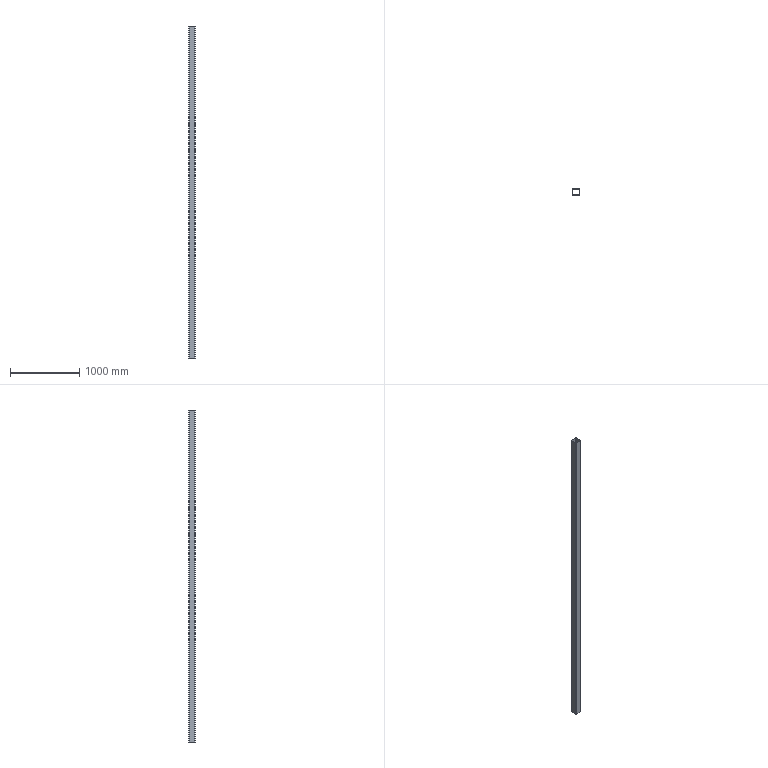Part | SolidWorks | features Extrusion 1 | 1 solid | 18 faces | box 100 x 100 x 4800 mm | volume 8810973 mm3 | plane 10 | cylinder 8 | commonest cylinder face diameters 10 x4 20 x4
STEP:
#1=CARTESIAN_POINT('',(-40.,50.,2400.));
#2=VERTEX_POINT('',#1);
#3=CARTESIAN_POINT('',(-50.,40.,2400.));
#4=VERTEX_POINT('',#3);
#5=CARTESIAN_POINT('',(-40.,40.,2400.));
#6=DIRECTION('',(0.,0.,1.));
#7=DIRECTION('',(1.,0.,0.));
#8=AXIS2_PLACEMENT_3D('',#5,#6,#7);
#9=CIRCLE('',#8,10.);
#10=EDGE_CURVE('',#2,#4,#9,.T.);
#11=ORIENTED_EDGE('',*,*,#10,.T.);
#12=CARTESIAN_POINT('',(-50.,-40.,2400.));
#13=VERTEX_POINT('',#12);
#14=CARTESIAN_POINT('',(-50.,40.,2400.));
#15=DIRECTION('',(0.,-1.,0.));
#16=VECTOR('',#15,1000.);
#17=LINE('',#14,#16);
#18=EDGE_CURVE('',#4,#13,#17,.T.);
#19=ORIENTED_EDGE('',*,*,#18,.T.);
#20=CARTESIAN_POINT('',(-40.,-50.,2400.));
#21=VERTEX_POINT('',#20);
#22=CARTESIAN_POINT('',(-40.,-40.,2400.));
#23=DIRECTION('',(0.,0.,1.));
#24=DIRECTION('',(-1.,0.,0.));
#25=AXIS2_PLACEMENT_3D('',#22,#23,#24);
#26=CIRCLE('',#25,10.);
#27=EDGE_CURVE('',#13,#21,#26,.T.);
#28=ORIENTED_EDGE('',*,*,#27,.T.);
#29=CARTESIAN_POINT('',(40.,-50.,2400.));
#30=VERTEX_POINT('',#29);
#31=CARTESIAN_POINT('',(40.,-50.,2400.));
#32=DIRECTION('',(1.,0.,0.));
#33=VECTOR('',#32,1000.);
#34=LINE('',#31,#33);
#35=EDGE_CURVE('',#21,#30,#34,.T.);
#36=ORIENTED_EDGE('',*,*,#35,.T.);
#37=CARTESIAN_POINT('',(50.,-40.,2400.));
#38=VERTEX_POINT('',#37);
#39=CARTESIAN_POINT('',(40.,-40.,2400.));
#40=DIRECTION('',(0.,0.,1.));
#41=DIRECTION('',(1.,0.,0.));
#42=AXIS2_PLACEMENT_3D('',#39,#40,#41);
#43=CIRCLE('',#42,10.);
#44=EDGE_CURVE('',#30,#38,#43,.T.);
#45=ORIENTED_EDGE('',*,*,#44,.T.);
#46=CARTESIAN_POINT('',(50.,40.,2400.));
#47=VERTEX_POINT('',#46);
#48=CARTESIAN_POINT('',(50.,-40.,2400.));
#49=DIRECTION('',(0.,1.,0.));
#50=VECTOR('',#49,1000.);
#51=LINE('',#48,#50);
#52=EDGE_CURVE('',#38,#47,#51,.T.);
#53=ORIENTED_EDGE('',*,*,#52,.T.);
#54=CARTESIAN_POINT('',(40.,50.,2400.));
#55=VERTEX_POINT('',#54);
#56=CARTESIAN_POINT('',(40.,40.,2400.));
#57=DIRECTION('',(0.,0.,1.));
#58=DIRECTION('',(-1.,0.,0.));
#59=AXIS2_PLACEMENT_3D('',#56,#57,#58);
#60=CIRCLE('',#59,10.);
#61=EDGE_CURVE('',#47,#55,#60,.T.);
#62=ORIENTED_EDGE('',*,*,#61,.T.);
#63=CARTESIAN_POINT('',(0.,50.,2400.));
#64=DIRECTION('',(-1.,0.,0.));
#65=VECTOR('',#64,1000.);
#66=LINE('',#63,#65);
#67=EDGE_CURVE('',#55,#2,#66,.T.);
#68=ORIENTED_EDGE('',*,*,#67,.T.);
#69=EDGE_LOOP('',(#11,#19,#28,#36,#45,#53,#62,#68));
#70=FACE_OUTER_BOUND('',#69,.T.);
#71=CARTESIAN_POINT('',(-45.,40.,2400.));
#72=VERTEX_POINT('',#71);
#73=CARTESIAN_POINT('',(-45.,-40.,2400.));
#74=VERTEX_POINT('',#73);
#75=CARTESIAN_POINT('',(-45.,40.,2400.));
#76=DIRECTION('',(0.,-1.,0.));
#77=VECTOR('',#76,1000.);
#78=LINE('',#75,#77);
#79=EDGE_CURVE('',#72,#74,#78,.T.);
#80=ORIENTED_EDGE('',*,*,#79,.F.);
#81=CARTESIAN_POINT('',(-40.,45.,2400.));
#82=VERTEX_POINT('',#81);
#83=CARTESIAN_POINT('',(-40.,40.,2400.));
#84=DIRECTION('',(0.,0.,1.));
#85=DIRECTION('',(1.,0.,0.));
#86=AXIS2_PLACEMENT_3D('',#83,#84,#85);
#87=CIRCLE('',#86,5.);
#88=EDGE_CURVE('',#82,#72,#87,.T.);
#89=ORIENTED_EDGE('',*,*,#88,.F.);
#90=CARTESIAN_POINT('',(40.,45.,2400.));
#91=VERTEX_POINT('',#90);
#92=CARTESIAN_POINT('',(0.,45.,2400.));
#93=DIRECTION('',(-1.,0.,0.));
#94=VECTOR('',#93,1000.);
#95=LINE('',#92,#94);
#96=EDGE_CURVE('',#91,#82,#95,.T.);
#97=ORIENTED_EDGE('',*,*,#96,.F.);
#98=CARTESIAN_POINT('',(45.,40.,2400.));
#99=VERTEX_POINT('',#98);
#100=CARTESIAN_POINT('',(40.,40.,2400.));
#101=DIRECTION('',(0.,0.,1.));
#102=DIRECTION('',(-1.,0.,0.));
#103=AXIS2_PLACEMENT_3D('',#100,#101,#102);
#104=CIRCLE('',#103,5.);
#105=EDGE_CURVE('',#99,#91,#104,.T.);
#106=ORIENTED_EDGE('',*,*,#105,.F.);
#107=CARTESIAN_POINT('',(45.,-40.,2400.));
#108=VERTEX_POINT('',#107);
#109=CARTESIAN_POINT('',(45.,-40.,2400.));
#110=DIRECTION('',(0.,1.,0.));
#111=VECTOR('',#110,1000.);
#112=LINE('',#109,#111);
#113=EDGE_CURVE('',#108,#99,#112,.T.);
#114=ORIENTED_EDGE('',*,*,#113,.F.);
#115=CARTESIAN_POINT('',(40.,-45.,2400.));
#116=VERTEX_POINT('',#115);
#117=CARTESIAN_POINT('',(40.,-40.,2400.));
#118=DIRECTION('',(0.,0.,1.));
#119=DIRECTION('',(1.,0.,0.));
#120=AXIS2_PLACEMENT_3D('',#117,#118,#119);
#121=CIRCLE('',#120,5.);
#122=EDGE_CURVE('',#116,#108,#121,.T.);
#123=ORIENTED_EDGE('',*,*,#122,.F.);
#124=CARTESIAN_POINT('',(-40.,-45.,2400.));
#125=VERTEX_POINT('',#124);
#126=CARTESIAN_POINT('',(40.,-45.,2400.));
#127=DIRECTION('',(1.,0.,0.));
#128=VECTOR('',#127,1000.);
#129=LINE('',#126,#128);
#130=EDGE_CURVE('',#125,#116,#129,.T.);
#131=ORIENTED_EDGE('',*,*,#130,.F.);
#132=CARTESIAN_POINT('',(-40.,-40.,2400.));
#133=DIRECTION('',(0.,0.,1.));
#134=DIRECTION('',(-1.,0.,0.));
#135=AXIS2_PLACEMENT_3D('',#132,#133,#134);
#136=CIRCLE('',#135,5.);
#137=EDGE_CURVE('',#74,#125,#136,.T.);
#138=ORIENTED_EDGE('',*,*,#137,.F.);
#139=EDGE_LOOP('',(#80,#89,#97,#106,#114,#123,#131,#138));
#140=FACE_BOUND('',#139,.T.);
#141=CARTESIAN_POINT('',(-40.,40.,2400.));
#142=DIRECTION('',(0.,0.,1.));
#143=DIRECTION('',(1.,0.,0.));
#144=AXIS2_PLACEMENT_3D('',#141,#142,#143);
#145=PLANE('',#144);
#146=ADVANCED_FACE('',(#70,#140),#145,.T.);
#147=CARTESIAN_POINT('',(-40.,50.,-2400.));
#148=VERTEX_POINT('',#147);
#149=CARTESIAN_POINT('',(-50.,40.,-2400.));
#150=VERTEX_POINT('',#149);
#151=CARTESIAN_POINT('',(-40.,40.,-2400.));
#152=DIRECTION('',(0.,0.,1.));
#153=DIRECTION('',(1.,0.,0.));
#154=AXIS2_PLACEMENT_3D('',#151,#152,#153);
#155=CIRCLE('',#154,10.);
#156=EDGE_CURVE('',#148,#150,#155,.T.);
#157=ORIENTED_EDGE('',*,*,#156,.F.);
#158=CARTESIAN_POINT('',(40.,50.,-2400.));
#159=VERTEX_POINT('',#158);
#160=CARTESIAN_POINT('',(0.,50.,-2400.));
#161=DIRECTION('',(-1.,0.,0.));
#162=VECTOR('',#161,1000.);
#163=LINE('',#160,#162);
#164=EDGE_CURVE('',#159,#148,#163,.T.);
#165=ORIENTED_EDGE('',*,*,#164,.F.);
#166=CARTESIAN_POINT('',(50.,40.,-2400.));
#167=VERTEX_POINT('',#166);
#168=CARTESIAN_POINT('',(40.,40.,-2400.));
#169=DIRECTION('',(0.,0.,1.));
#170=DIRECTION('',(-1.,0.,0.));
#171=AXIS2_PLACEMENT_3D('',#168,#169,#170);
#172=CIRCLE('',#171,10.);
#173=EDGE_CURVE('',#167,#159,#172,.T.);
#174=ORIENTED_EDGE('',*,*,#173,.F.);
#175=CARTESIAN_POINT('',(50.,-40.,-2400.));
#176=VERTEX_POINT('',#175);
#177=CARTESIAN_POINT('',(50.,40.,-2400.));
#178=DIRECTION('',(0.,1.,0.));
#179=VECTOR('',#178,1000.);
#180=LINE('',#177,#179);
#181=EDGE_CURVE('',#176,#167,#180,.T.);
#182=ORIENTED_EDGE('',*,*,#181,.F.);
#183=CARTESIAN_POINT('',(40.,-50.,-2400.));
#184=VERTEX_POINT('',#183);
#185=CARTESIAN_POINT('',(40.,-40.,-2400.));
#186=DIRECTION('',(0.,0.,1.));
#187=DIRECTION('',(1.,0.,0.));
#188=AXIS2_PLACEMENT_3D('',#185,#186,#187);
#189=CIRCLE('',#188,10.);
#190=EDGE_CURVE('',#184,#176,#189,.T.);
#191=ORIENTED_EDGE('',*,*,#190,.F.);
#192=CARTESIAN_POINT('',(-40.,-50.,-2400.));
#193=VERTEX_POINT('',#192);
#194=CARTESIAN_POINT('',(40.,-50.,-2400.));
#195=DIRECTION('',(1.,0.,0.));
#196=VECTOR('',#195,1000.);
#197=LINE('',#194,#196);
#198=EDGE_CURVE('',#193,#184,#197,.T.);
#199=ORIENTED_EDGE('',*,*,#198,.F.);
#200=CARTESIAN_POINT('',(-50.,-40.,-2400.));
#201=VERTEX_POINT('',#200);
#202=CARTESIAN_POINT('',(-40.,-40.,-2400.));
#203=DIRECTION('',(0.,0.,1.));
#204=DIRECTION('',(-1.,0.,0.));
#205=AXIS2_PLACEMENT_3D('',#202,#203,#204);
#206=CIRCLE('',#205,10.);
#207=EDGE_CURVE('',#201,#193,#206,.T.);
#208=ORIENTED_EDGE('',*,*,#207,.F.);
#209=CARTESIAN_POINT('',(-50.,-40.,-2400.));
#210=DIRECTION('',(0.,-1.,0.));
#211=VECTOR('',#210,1000.);
#212=LINE('',#209,#211);
#213=EDGE_CURVE('',#150,#201,#212,.T.);
#214=ORIENTED_EDGE('',*,*,#213,.F.);
#215=EDGE_LOOP('',(#157,#165,#174,#182,#191,#199,#208,#214));
#216=FACE_OUTER_BOUND('',#215,.T.);
#217=CARTESIAN_POINT('',(-40.,45.,-2400.));
#218=VERTEX_POINT('',#217);
#219=CARTESIAN_POINT('',(-45.,40.,-2400.));
#220=VERTEX_POINT('',#219);
#221=CARTESIAN_POINT('',(-40.,40.,-2400.));
#222=DIRECTION('',(0.,0.,1.));
#223=DIRECTION('',(1.,0.,0.));
#224=AXIS2_PLACEMENT_3D('',#221,#222,#223);
#225=CIRCLE('',#224,5.);
#226=EDGE_CURVE('',#218,#220,#225,.T.);
#227=ORIENTED_EDGE('',*,*,#226,.T.);
#228=CARTESIAN_POINT('',(-45.,-40.,-2400.));
#229=VERTEX_POINT('',#228);
#230=CARTESIAN_POINT('',(-45.,-40.,-2400.));
#231=DIRECTION('',(0.,-1.,0.));
#232=VECTOR('',#231,1000.);
#233=LINE('',#230,#232);
#234=EDGE_CURVE('',#220,#229,#233,.T.);
#235=ORIENTED_EDGE('',*,*,#234,.T.);
#236=CARTESIAN_POINT('',(-40.,-45.,-2400.));
#237=VERTEX_POINT('',#236);
#238=CARTESIAN_POINT('',(-40.,-40.,-2400.));
#239=DIRECTION('',(0.,0.,1.));
#240=DIRECTION('',(-1.,0.,0.));
#241=AXIS2_PLACEMENT_3D('',#238,#239,#240);
#242=CIRCLE('',#241,5.);
#243=EDGE_CURVE('',#229,#237,#242,.T.);
#244=ORIENTED_EDGE('',*,*,#243,.T.);
#245=CARTESIAN_POINT('',(40.,-45.,-2400.));
#246=VERTEX_POINT('',#245);
#247=CARTESIAN_POINT('',(40.,-45.,-2400.));
#248=DIRECTION('',(1.,0.,0.));
#249=VECTOR('',#248,1000.);
#250=LINE('',#247,#249);
#251=EDGE_CURVE('',#237,#246,#250,.T.);
#252=ORIENTED_EDGE('',*,*,#251,.T.);
#253=CARTESIAN_POINT('',(45.,-40.,-2400.));
#254=VERTEX_POINT('',#253);
#255=CARTESIAN_POINT('',(40.,-40.,-2400.));
#256=DIRECTION('',(0.,0.,1.));
#257=DIRECTION('',(1.,0.,0.));
#258=AXIS2_PLACEMENT_3D('',#255,#256,#257);
#259=CIRCLE('',#258,5.);
#260=EDGE_CURVE('',#246,#254,#259,.T.);
#261=ORIENTED_EDGE('',*,*,#260,.T.);
#262=CARTESIAN_POINT('',(45.,40.,-2400.));
#263=VERTEX_POINT('',#262);
#264=CARTESIAN_POINT('',(45.,40.,-2400.));
#265=DIRECTION('',(0.,1.,0.));
#266=VECTOR('',#265,1000.);
#267=LINE('',#264,#266);
#268=EDGE_CURVE('',#254,#263,#267,.T.);
#269=ORIENTED_EDGE('',*,*,#268,.T.);
#270=CARTESIAN_POINT('',(40.,45.,-2400.));
#271=VERTEX_POINT('',#270);
#272=CARTESIAN_POINT('',(40.,40.,-2400.));
#273=DIRECTION('',(0.,0.,1.));
#274=DIRECTION('',(-1.,0.,0.));
#275=AXIS2_PLACEMENT_3D('',#272,#273,#274);
#276=CIRCLE('',#275,5.);
#277=EDGE_CURVE('',#263,#271,#276,.T.);
#278=ORIENTED_EDGE('',*,*,#277,.T.);
#279=CARTESIAN_POINT('',(0.,45.,-2400.));
#280=DIRECTION('',(-1.,0.,0.));
#281=VECTOR('',#280,1000.);
#282=LINE('',#279,#281);
#283=EDGE_CURVE('',#271,#218,#282,.T.);
#284=ORIENTED_EDGE('',*,*,#283,.T.);
#285=EDGE_LOOP('',(#227,#235,#244,#252,#261,#269,#278,#284));
#286=FACE_BOUND('',#285,.T.);
#287=CARTESIAN_POINT('',(-40.,40.,-2400.));
#288=DIRECTION('',(0.,0.,1.));
#289=DIRECTION('',(1.,0.,0.));
#290=AXIS2_PLACEMENT_3D('',#287,#288,#289);
#291=PLANE('',#290);
#292=ADVANCED_FACE('',(#216,#286),#291,.F.);
#293=ORIENTED_EDGE('',*,*,#156,.T.);
#294=CARTESIAN_POINT('',(-50.,40.,2400.));
#295=DIRECTION('',(0.,0.,-1.));
#296=VECTOR('',#295,1000.);
#297=LINE('',#294,#296);
#298=EDGE_CURVE('',#4,#150,#297,.T.);
#299=ORIENTED_EDGE('',*,*,#298,.F.);
#300=ORIENTED_EDGE('',*,*,#10,.F.);
#301=CARTESIAN_POINT('',(-40.,50.,2400.));
#302=DIRECTION('',(0.,0.,-1.));
#303=VECTOR('',#302,1000.);
#304=LINE('',#301,#303);
#305=EDGE_CURVE('',#2,#148,#304,.T.);
#306=ORIENTED_EDGE('',*,*,#305,.T.);
#307=EDGE_LOOP('',(#293,#299,#300,#306));
#308=FACE_OUTER_BOUND('',#307,.T.);
#309=CARTESIAN_POINT('',(-40.,40.,2400.));
#310=DIRECTION('',(0.,0.,-1.));
#311=DIRECTION('',(-1.,0.,0.));
#312=AXIS2_PLACEMENT_3D('',#309,#310,#311);
#313=CYLINDRICAL_SURFACE('',#312,10.);
#314=ADVANCED_FACE('',(#308),#313,.T.);
#315=ORIENTED_EDGE('',*,*,#213,.T.);
#316=CARTESIAN_POINT('',(-50.,-40.,2400.));
#317=DIRECTION('',(0.,0.,-1.));
#318=VECTOR('',#317,1000.);
#319=LINE('',#316,#318);
#320=EDGE_CURVE('',#13,#201,#319,.T.);
#321=ORIENTED_EDGE('',*,*,#320,.F.);
#322=ORIENTED_EDGE('',*,*,#18,.F.);
#323=ORIENTED_EDGE('',*,*,#298,.T.);
#324=EDGE_LOOP('',(#315,#321,#322,#323));
#325=FACE_OUTER_BOUND('',#324,.T.);
#326=CARTESIAN_POINT('',(-50.,-40.,2400.));
#327=DIRECTION('',(1.,0.,0.));
#328=DIRECTION('',(0.,1.,0.));
#329=AXIS2_PLACEMENT_3D('',#326,#327,#328);
#330=PLANE('',#329);
#331=ADVANCED_FACE('',(#325),#330,.F.);
#332=ORIENTED_EDGE('',*,*,#207,.T.);
#333=CARTESIAN_POINT('',(-40.,-50.,2400.));
#334=DIRECTION('',(0.,0.,-1.));
#335=VECTOR('',#334,1000.);
#336=LINE('',#333,#335);
#337=EDGE_CURVE('',#21,#193,#336,.T.);
#338=ORIENTED_EDGE('',*,*,#337,.F.);
#339=ORIENTED_EDGE('',*,*,#27,.F.);
#340=ORIENTED_EDGE('',*,*,#320,.T.);
#341=EDGE_LOOP('',(#332,#338,#339,#340));
#342=FACE_OUTER_BOUND('',#341,.T.);
#343=CARTESIAN_POINT('',(-40.,-40.,2400.));
#344=DIRECTION('',(0.,0.,-1.));
#345=DIRECTION('',(-1.,0.,0.));
#346=AXIS2_PLACEMENT_3D('',#343,#344,#345);
#347=CYLINDRICAL_SURFACE('',#346,10.);
#348=ADVANCED_FACE('',(#342),#347,.T.);
#349=ORIENTED_EDGE('',*,*,#198,.T.);
#350=CARTESIAN_POINT('',(40.,-50.,2400.));
#351=DIRECTION('',(0.,0.,-1.));
#352=VECTOR('',#351,1000.);
#353=LINE('',#350,#352);
#354=EDGE_CURVE('',#30,#184,#353,.T.);
#355=ORIENTED_EDGE('',*,*,#354,.F.);
#356=ORIENTED_EDGE('',*,*,#35,.F.);
#357=ORIENTED_EDGE('',*,*,#337,.T.);
#358=EDGE_LOOP('',(#349,#355,#356,#357));
#359=FACE_OUTER_BOUND('',#358,.T.);
#360=CARTESIAN_POINT('',(40.,-50.,2400.));
#361=DIRECTION('',(0.,1.,0.));
#362=DIRECTION('',(-1.,0.,0.));
#363=AXIS2_PLACEMENT_3D('',#360,#361,#362);
#364=PLANE('',#363);
#365=ADVANCED_FACE('',(#359),#364,.F.);
#366=ORIENTED_EDGE('',*,*,#190,.T.);
#367=CARTESIAN_POINT('',(50.,-40.,2400.));
#368=DIRECTION('',(0.,0.,-1.));
#369=VECTOR('',#368,1000.);
#370=LINE('',#367,#369);
#371=EDGE_CURVE('',#38,#176,#370,.T.);
#372=ORIENTED_EDGE('',*,*,#371,.F.);
#373=ORIENTED_EDGE('',*,*,#44,.F.);
#374=ORIENTED_EDGE('',*,*,#354,.T.);
#375=EDGE_LOOP('',(#366,#372,#373,#374));
#376=FACE_OUTER_BOUND('',#375,.T.);
#377=CARTESIAN_POINT('',(40.,-40.,2400.));
#378=DIRECTION('',(0.,0.,-1.));
#379=DIRECTION('',(-1.,0.,0.));
#380=AXIS2_PLACEMENT_3D('',#377,#378,#379);
#381=CYLINDRICAL_SURFACE('',#380,10.);
#382=ADVANCED_FACE('',(#376),#381,.T.);
#383=ORIENTED_EDGE('',*,*,#181,.T.);
#384=CARTESIAN_POINT('',(50.,40.,2400.));
#385=DIRECTION('',(0.,0.,-1.));
#386=VECTOR('',#385,1000.);
#387=LINE('',#384,#386);
#388=EDGE_CURVE('',#47,#167,#387,.T.);
#389=ORIENTED_EDGE('',*,*,#388,.F.);
#390=ORIENTED_EDGE('',*,*,#52,.F.);
#391=ORIENTED_EDGE('',*,*,#371,.T.);
#392=EDGE_LOOP('',(#383,#389,#390,#391));
#393=FACE_OUTER_BOUND('',#392,.T.);
#394=CARTESIAN_POINT('',(50.,40.,2400.));
#395=DIRECTION('',(-1.,0.,0.));
#396=DIRECTION('',(0.,-1.,0.));
#397=AXIS2_PLACEMENT_3D('',#394,#395,#396);
#398=PLANE('',#397);
#399=ADVANCED_FACE('',(#393),#398,.F.);
#400=ORIENTED_EDGE('',*,*,#173,.T.);
#401=CARTESIAN_POINT('',(40.,50.,2400.));
#402=DIRECTION('',(0.,0.,-1.));
#403=VECTOR('',#402,1000.);
#404=LINE('',#401,#403);
#405=EDGE_CURVE('',#55,#159,#404,.T.);
#406=ORIENTED_EDGE('',*,*,#405,.F.);
#407=ORIENTED_EDGE('',*,*,#61,.F.);
#408=ORIENTED_EDGE('',*,*,#388,.T.);
#409=EDGE_LOOP('',(#400,#406,#407,#408));
#410=FACE_OUTER_BOUND('',#409,.T.);
#411=CARTESIAN_POINT('',(40.,40.,2400.));
#412=DIRECTION('',(0.,0.,-1.));
#413=DIRECTION('',(-1.,0.,0.));
#414=AXIS2_PLACEMENT_3D('',#411,#412,#413);
#415=CYLINDRICAL_SURFACE('',#414,10.);
#416=ADVANCED_FACE('',(#410),#415,.T.);
#417=ORIENTED_EDGE('',*,*,#164,.T.);
#418=ORIENTED_EDGE('',*,*,#305,.F.);
#419=ORIENTED_EDGE('',*,*,#67,.F.);
#420=ORIENTED_EDGE('',*,*,#405,.T.);
#421=EDGE_LOOP('',(#417,#418,#419,#420));
#422=FACE_OUTER_BOUND('',#421,.T.);
#423=CARTESIAN_POINT('',(0.,50.,2400.));
#424=DIRECTION('',(0.,-1.,0.));
#425=DIRECTION('',(1.,0.,0.));
#426=AXIS2_PLACEMENT_3D('',#423,#424,#425);
#427=PLANE('',#426);
#428=ADVANCED_FACE('',(#422),#427,.F.);
#429=ORIENTED_EDGE('',*,*,#226,.F.);
#430=CARTESIAN_POINT('',(-40.,45.,2400.));
#431=DIRECTION('',(0.,0.,-1.));
#432=VECTOR('',#431,1000.);
#433=LINE('',#430,#432);
#434=EDGE_CURVE('',#82,#218,#433,.T.);
#435=ORIENTED_EDGE('',*,*,#434,.F.);
#436=ORIENTED_EDGE('',*,*,#88,.T.);
#437=CARTESIAN_POINT('',(-45.,40.,2400.));
#438=DIRECTION('',(0.,0.,-1.));
#439=VECTOR('',#438,1000.);
#440=LINE('',#437,#439);
#441=EDGE_CURVE('',#72,#220,#440,.T.);
#442=ORIENTED_EDGE('',*,*,#441,.T.);
#443=EDGE_LOOP('',(#429,#435,#436,#442));
#444=FACE_OUTER_BOUND('',#443,.T.);
#445=CARTESIAN_POINT('',(-40.,40.,2400.));
#446=DIRECTION('',(0.,0.,-1.));
#447=DIRECTION('',(-1.,0.,0.));
#448=AXIS2_PLACEMENT_3D('',#445,#446,#447);
#449=CYLINDRICAL_SURFACE('',#448,5.);
#450=ADVANCED_FACE('',(#444),#449,.F.);
#451=ORIENTED_EDGE('',*,*,#234,.F.);
#452=ORIENTED_EDGE('',*,*,#441,.F.);
#453=ORIENTED_EDGE('',*,*,#79,.T.);
#454=CARTESIAN_POINT('',(-45.,-40.,2400.));
#455=DIRECTION('',(0.,0.,-1.));
#456=VECTOR('',#455,1000.);
#457=LINE('',#454,#456);
#458=EDGE_CURVE('',#74,#229,#457,.T.);
#459=ORIENTED_EDGE('',*,*,#458,.T.);
#460=EDGE_LOOP('',(#451,#452,#453,#459));
#461=FACE_OUTER_BOUND('',#460,.T.);
#462=CARTESIAN_POINT('',(-45.,-40.,2400.));
#463=DIRECTION('',(1.,0.,0.));
#464=DIRECTION('',(0.,0.,-1.));
#465=AXIS2_PLACEMENT_3D('',#462,#463,#464);
#466=PLANE('',#465);
#467=ADVANCED_FACE('',(#461),#466,.T.);
#468=ORIENTED_EDGE('',*,*,#243,.F.);
#469=ORIENTED_EDGE('',*,*,#458,.F.);
#470=ORIENTED_EDGE('',*,*,#137,.T.);
#471=CARTESIAN_POINT('',(-40.,-45.,2400.));
#472=DIRECTION('',(0.,0.,-1.));
#473=VECTOR('',#472,1000.);
#474=LINE('',#471,#473);
#475=EDGE_CURVE('',#125,#237,#474,.T.);
#476=ORIENTED_EDGE('',*,*,#475,.T.);
#477=EDGE_LOOP('',(#468,#469,#470,#476));
#478=FACE_OUTER_BOUND('',#477,.T.);
#479=CARTESIAN_POINT('',(-40.,-40.,2400.));
#480=DIRECTION('',(0.,0.,-1.));
#481=DIRECTION('',(-1.,0.,0.));
#482=AXIS2_PLACEMENT_3D('',#479,#480,#481);
#483=CYLINDRICAL_SURFACE('',#482,5.);
#484=ADVANCED_FACE('',(#478),#483,.F.);
#485=ORIENTED_EDGE('',*,*,#251,.F.);
#486=ORIENTED_EDGE('',*,*,#475,.F.);
#487=ORIENTED_EDGE('',*,*,#130,.T.);
#488=CARTESIAN_POINT('',(40.,-45.,2400.));
#489=DIRECTION('',(0.,0.,-1.));
#490=VECTOR('',#489,1000.);
#491=LINE('',#488,#490);
#492=EDGE_CURVE('',#116,#246,#491,.T.);
#493=ORIENTED_EDGE('',*,*,#492,.T.);
#494=EDGE_LOOP('',(#485,#486,#487,#493));
#495=FACE_OUTER_BOUND('',#494,.T.);
#496=CARTESIAN_POINT('',(40.,-45.,2400.));
#497=DIRECTION('',(0.,1.,0.));
#498=DIRECTION('',(-1.,0.,0.));
#499=AXIS2_PLACEMENT_3D('',#496,#497,#498);
#500=PLANE('',#499);
#501=ADVANCED_FACE('',(#495),#500,.T.);
#502=ORIENTED_EDGE('',*,*,#260,.F.);
#503=ORIENTED_EDGE('',*,*,#492,.F.);
#504=ORIENTED_EDGE('',*,*,#122,.T.);
#505=CARTESIAN_POINT('',(45.,-40.,2400.));
#506=DIRECTION('',(0.,0.,-1.));
#507=VECTOR('',#506,1000.);
#508=LINE('',#505,#507);
#509=EDGE_CURVE('',#108,#254,#508,.T.);
#510=ORIENTED_EDGE('',*,*,#509,.T.);
#511=EDGE_LOOP('',(#502,#503,#504,#510));
#512=FACE_OUTER_BOUND('',#511,.T.);
#513=CARTESIAN_POINT('',(40.,-40.,2400.));
#514=DIRECTION('',(0.,0.,-1.));
#515=DIRECTION('',(-1.,0.,0.));
#516=AXIS2_PLACEMENT_3D('',#513,#514,#515);
#517=CYLINDRICAL_SURFACE('',#516,5.);
#518=ADVANCED_FACE('',(#512),#517,.F.);
#519=ORIENTED_EDGE('',*,*,#268,.F.);
#520=ORIENTED_EDGE('',*,*,#509,.F.);
#521=ORIENTED_EDGE('',*,*,#113,.T.);
#522=CARTESIAN_POINT('',(45.,40.,2400.));
#523=DIRECTION('',(0.,0.,-1.));
#524=VECTOR('',#523,1000.);
#525=LINE('',#522,#524);
#526=EDGE_CURVE('',#99,#263,#525,.T.);
#527=ORIENTED_EDGE('',*,*,#526,.T.);
#528=EDGE_LOOP('',(#519,#520,#521,#527));
#529=FACE_OUTER_BOUND('',#528,.T.);
#530=CARTESIAN_POINT('',(45.,40.,2400.));
#531=DIRECTION('',(-1.,0.,0.));
#532=DIRECTION('',(0.,0.,1.));
#533=AXIS2_PLACEMENT_3D('',#530,#531,#532);
#534=PLANE('',#533);
#535=ADVANCED_FACE('',(#529),#534,.T.);
#536=ORIENTED_EDGE('',*,*,#277,.F.);
#537=ORIENTED_EDGE('',*,*,#526,.F.);
#538=ORIENTED_EDGE('',*,*,#105,.T.);
#539=CARTESIAN_POINT('',(40.,45.,2400.));
#540=DIRECTION('',(0.,0.,-1.));
#541=VECTOR('',#540,1000.);
#542=LINE('',#539,#541);
#543=EDGE_CURVE('',#91,#271,#542,.T.);
#544=ORIENTED_EDGE('',*,*,#543,.T.);
#545=EDGE_LOOP('',(#536,#537,#538,#544));
#546=FACE_OUTER_BOUND('',#545,.T.);
#547=CARTESIAN_POINT('',(40.,40.,2400.));
#548=DIRECTION('',(0.,0.,-1.));
#549=DIRECTION('',(-1.,0.,0.));
#550=AXIS2_PLACEMENT_3D('',#547,#548,#549);
#551=CYLINDRICAL_SURFACE('',#550,5.);
#552=ADVANCED_FACE('',(#546),#551,.F.);
#553=ORIENTED_EDGE('',*,*,#283,.F.);
#554=ORIENTED_EDGE('',*,*,#543,.F.);
#555=ORIENTED_EDGE('',*,*,#96,.T.);
#556=ORIENTED_EDGE('',*,*,#434,.T.);
#557=EDGE_LOOP('',(#553,#554,#555,#556));
#558=FACE_OUTER_BOUND('',#557,.T.);
#559=CARTESIAN_POINT('',(0.,45.,2400.));
#560=DIRECTION('',(0.,-1.,0.));
#561=DIRECTION('',(1.,0.,0.));
#562=AXIS2_PLACEMENT_3D('',#559,#560,#561);
#563=PLANE('',#562);
#564=ADVANCED_FACE('',(#558),#563,.T.);
#565=CLOSED_SHELL('',(#146,#292,#314,#331,#348,#365,#382,#399,#416,#428,#450,#467,#484,#501,#518,#535,#552,#564));
#566=MANIFOLD_SOLID_BREP('',#565);
#567=CARTESIAN_POINT('',(0.,0.,0.));
#568=DIRECTION('',(0.,0.,1.));
#569=DIRECTION('',(1.,0.,0.));
#570=AXIS2_PLACEMENT_3D('',#567,#568,#569);
#571=(LENGTH_UNIT()NAMED_UNIT(*)SI_UNIT(.MILLI.,.METRE.));
#572=UNCERTAINTY_MEASURE_WITH_UNIT(LENGTH_MEASURE(0.00001),#571,'','');
#573=(NAMED_UNIT(*)PLANE_ANGLE_UNIT()SI_UNIT($,.RADIAN.));
#574=(NAMED_UNIT(*)SI_UNIT($,.STERADIAN.)SOLID_ANGLE_UNIT());
#575=(GEOMETRIC_REPRESENTATION_CONTEXT(3)GLOBAL_UNCERTAINTY_ASSIGNED_CONTEXT((#572))GLOBAL_UNIT_ASSIGNED_CONTEXT((#571,#573,#574))REPRESENTATION_CONTEXT('',''));
#576=ADVANCED_BREP_SHAPE_REPRESENTATION('',(#566,#570),#575);